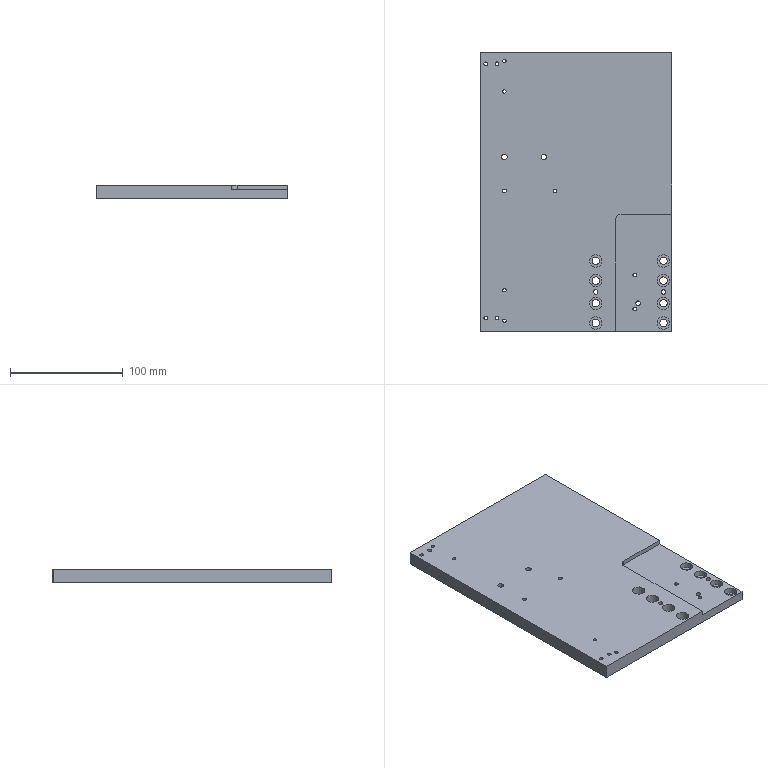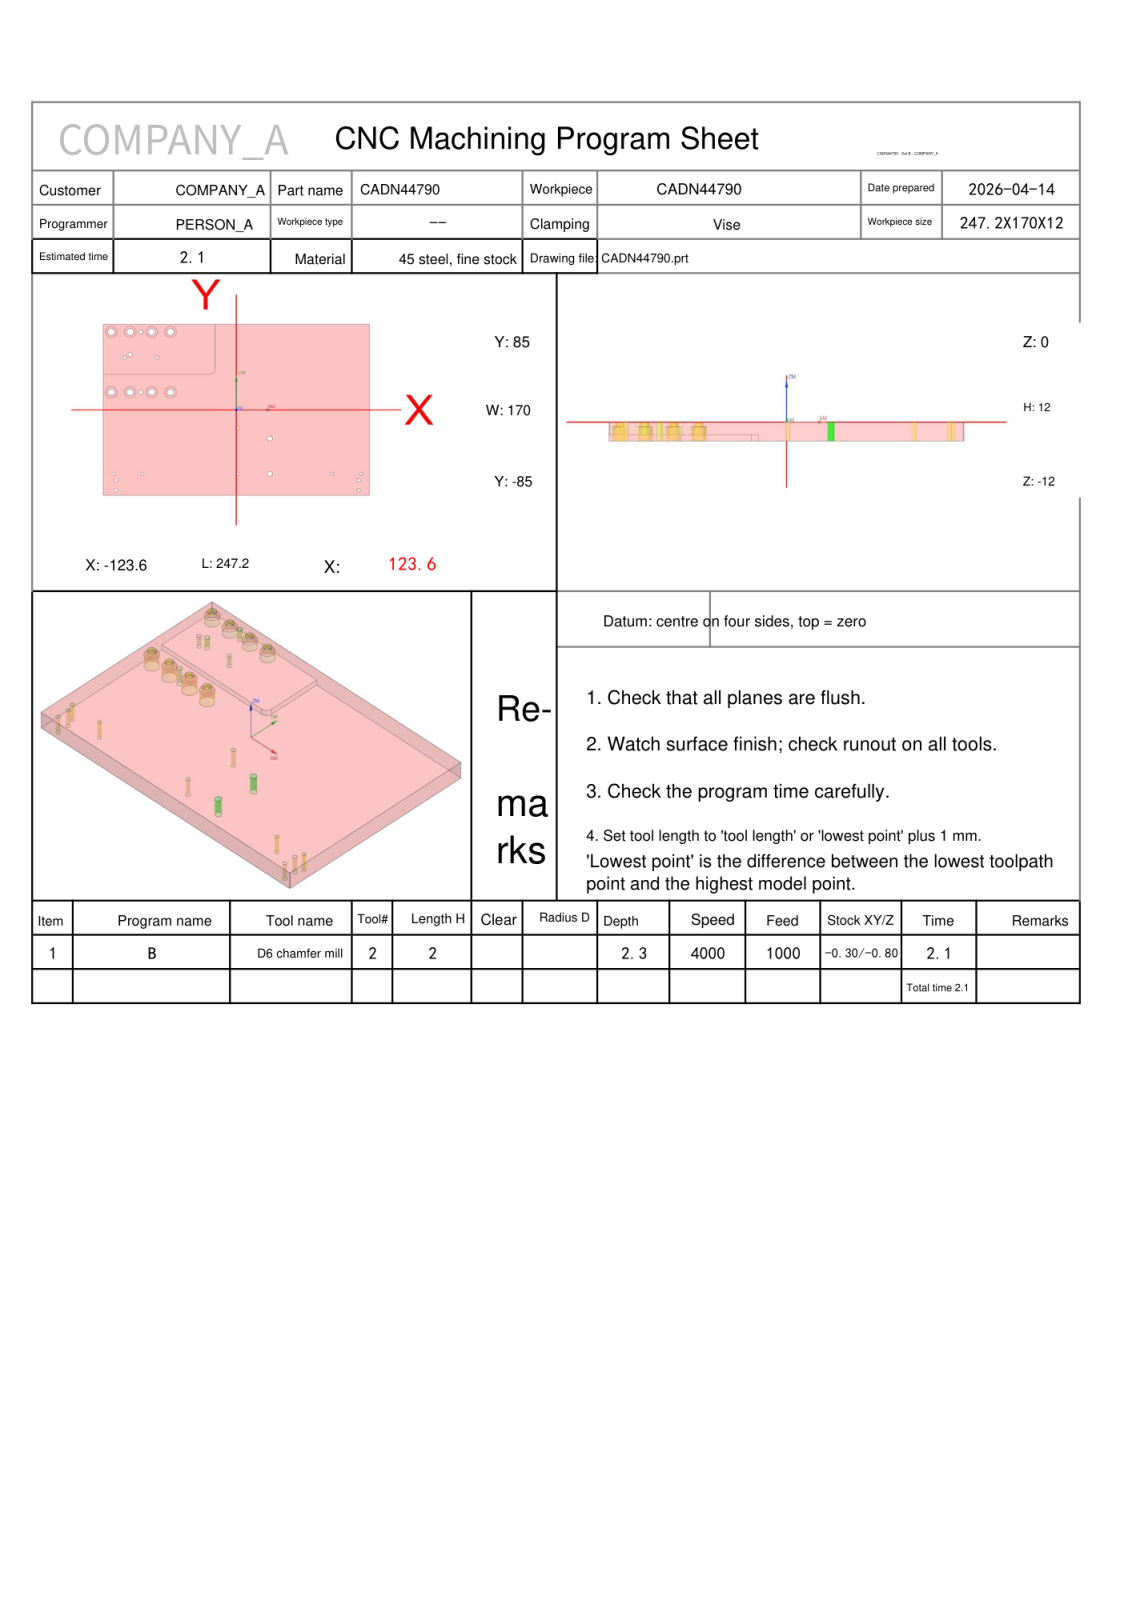NC program | NX | posted by the shop | part box 170 x 247.2 x 12 mm
Whole program:
%
O0001
(Machine time: 2.29 MIN)
(===Total Tool:1===)
(T2=D6 chamfer mill   D=6.   R=0.   D-  H02 Z=-2.3  )
G80 G90 G17 G49 G40
G91 G28 Z0
M01
N1 T02 M06
(D6 chamfer mill D=6. R=0. H=02 ce=0.00 di=0.00)
G00 G90 G54 X116.1 Y-63.5 M03 S2000
G43 H02 Z20.
M08
G98 G81 X116.1 Y-63.5 Z-1.8 R3. F100.
X89.1
X-87.1
X-114.1
G80
G00 Z20.
G00 G90 X-88.6 Y17.5 M03 S2000
Z20.
G98 G81 X-88.6 Y17.5 Z-2.3 R3. F100.
X-98.6 Y55.
X-88.6 Y77.5
G80
G00 Z20.
G00 G90 X113.6 Y-80. M03 S2000
Z20.
G98 G81 X113.6 Y-80. Z-2.2 R3. F100.
Y-70.
X1. Y-63.5
Y-18.5
X-73.6 Y52.
X-103.6
X-111.6 Y-70.
Y-80.
G80
G00 Z20.
G00 G90 X30.81 Y-63.563 M03 S4000
Z20.
Z-1.1
G01 Z-1.6 F600.
X30.776 Y-63.574
G03 X30.747 Y-63.867 I1.471 J-.293
X31. Y-64.7 I1.5 J0.0
X32.2 Y-63.5 I0.0 J1.2
X31. Y-62.3 I-1.2 J0.0
X29.8 Y-63.5 I0.0 J-1.2
X31. Y-64.7 I1.2 J0.0
X31.253 Y-63.867 I-1.247 J.833
X31.224 Y-63.574 I-1.5 J0.0
G01 X31.19 Y-63.563
Z-1.1
G00 Z20.
X30.81 Y-28.563
Z-1.1
G01 Z-1.6
X30.776 Y-28.574
G03 X30.747 Y-28.867 I1.471 J-.293
X31. Y-29.7 I1.5 J0.0
X32.2 Y-28.5 I0.0 J1.2
X31. Y-27.3 I-1.2 J0.0
X29.8 Y-28.5 I0.0 J-1.2
X31. Y-29.7 I1.2 J0.0
X31.253 Y-28.867 I-1.247 J.833
X31.224 Y-28.574 I-1.5 J0.0
G01 X31.19 Y-28.563
Z-1.1
G00 Z20.
G00 G90 X-117.049 Y17.184 M03 S4000
Z20.
Z-1.1
G01 Z-1.6 F600.
X-117.6 Y17.
G03 X-116.1 Y15.5 I1.5 J0.0
X-114.1 Y17.5 I0.0 J2.
X-116.1 Y19.5 I-2. J0.0
X-118.1 Y17.5 I0.0 J-2.
X-116.1 Y15.5 I2. J0.0
X-114.6 Y17. I0.0 J1.5
G01 X-115.151 Y17.184
Z-1.1
G00 Z20.
X-99.549
Z-1.1
G01 Z-1.6
X-100.1 Y17.
G03 X-98.6 Y15.5 I1.5 J0.0
X-96.6 Y17.5 I0.0 J2.
X-98.6 Y19.5 I-2. J0.0
X-100.6 Y17.5 I0.0 J-2.
X-98.6 Y15.5 I2. J0.0
X-97.1 Y17. I0.0 J1.5
G01 X-97.651 Y17.184
Z-1.1
G00 Z20.
X-79.549
Z-1.1
G01 Z-1.6
X-80.1 Y17.
G03 X-78.6 Y15.5 I1.5 J0.0
X-76.6 Y17.5 I0.0 J2.
X-78.6 Y19.5 I-2. J0.0
X-80.6 Y17.5 I0.0 J-2.
X-78.6 Y15.5 I2. J0.0
X-77.1 Y17. I0.0 J1.5
G01 X-77.651 Y17.184
Z-1.1
G00 Z20.
X-62.049
Z-1.1
G01 Z-1.6
X-62.6 Y17.
G03 X-61.1 Y15.5 I1.5 J0.0
X-59.1 Y17.5 I0.0 J2.
X-61.1 Y19.5 I-2. J0.0
X-63.1 Y17.5 I0.0 J-2.
X-61.1 Y15.5 I2. J0.0
X-59.6 Y17. I0.0 J1.5
G01 X-60.151 Y17.184
Z-1.1
G00 Z20.
X-62.049 Y77.184
Z-1.1
G01 Z-1.6
X-62.6 Y77.
G03 X-61.1 Y75.5 I1.5 J0.0
X-59.1 Y77.5 I0.0 J2.
X-61.1 Y79.5 I-2. J0.0
X-63.1 Y77.5 I0.0 J-2.
X-61.1 Y75.5 I2. J0.0
X-59.6 Y77. I0.0 J1.5
G01 X-60.151 Y77.184
Z-1.1
G00 Z20.
X-79.549
Z-1.1
G01 Z-1.6
X-80.1 Y77.
G03 X-78.6 Y75.5 I1.5 J0.0
X-76.6 Y77.5 I0.0 J2.
X-78.6 Y79.5 I-2. J0.0
X-80.6 Y77.5 I0.0 J-2.
X-78.6 Y75.5 I2. J0.0
X-77.1 Y77. I0.0 J1.5
G01 X-77.651 Y77.184
Z-1.1
G00 Z20.
X-99.549
Z-1.1
G01 Z-1.6
X-100.1 Y77.
G03 X-98.6 Y75.5 I1.5 J0.0
X-96.6 Y77.5 I0.0 J2.
X-98.6 Y79.5 I-2. J0.0
X-100.6 Y77.5 I0.0 J-2.
X-98.6 Y75.5 I2. J0.0
X-97.1 Y77. I0.0 J1.5
G01 X-97.651 Y77.184
Z-1.1
G00 Z20.
X-117.049
Z-1.1
G01 Z-1.6
X-117.6 Y77.
G03 X-116.1 Y75.5 I1.5 J0.0
X-114.1 Y77.5 I0.0 J2.
X-116.1 Y79.5 I-2. J0.0
X-118.1 Y77.5 I0.0 J-2.
X-116.1 Y75.5 I2. J0.0
X-114.6 Y77. I0.0 J1.5
G01 X-115.151 Y77.184
Z-1.1
G00 Z20.
G00 G90 X124.6 Y-74.958 M03 S4000
Z20.
Z2.5
G01 Y-84.464 Z-.96 F1000.
X124.569 Y-84.673 Z-1.037
X124.504 Y-84.874 Z-1.114
X124.407 Y-85.062 Z-1.191
X124.282 Y-85.232 Z-1.268
X124.219 Y-85.295 Z-1.3
X123.895 Y-85.619
G02 X122.976 Y-86. I-.919 J.919
G01 X-123.3
G02 X-124.6 Y-84.7 I0.0 J1.3
G01 Y84.376
G02 X-124.219 Y85.295 I1.3 J0.0
G01 X-123.895 Y85.619
G02 X-122.976 Y86. I.919 J-.919
G01 X123.3
G02 X124.6 Y84.7 I0.0 J-1.3
G01 Y-84.376
G02 X124.219 Y-85.295 I-1.3 J0.0
G01 X123.895 Y-85.619
X123.865 Y-85.648
Z1.2
G00 Z20.
M05
M09
G91 G28 Z0.0
G91 G28 Y0.0
M30
%